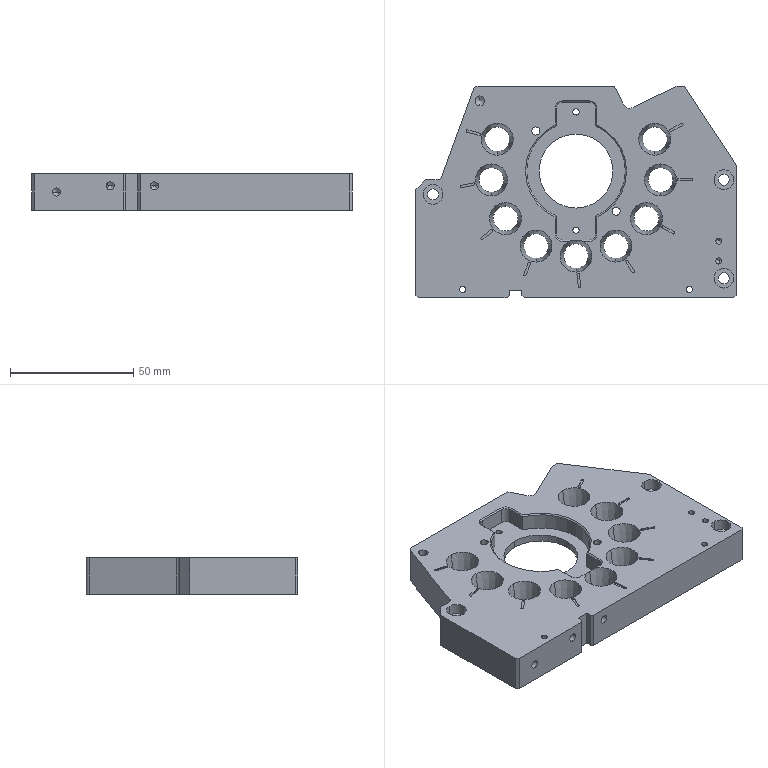NC program | NX | posted with a generic post | part box 130 x 86 x 15 mm
Lines 3983 to 5005 of 51277:
(ZLEVEL_PROFILE_1 , TOOL : D4)
N7898 T17 M6
N7900 G54
N7902 G17 G0 G90 X-13.91 Y5.2 B0. C0. S6500 M3
N7904 G43 Z30. H17
N7906 Z-0.6
N7908 G94 G1 X-14.257 Y5.8 F1650.
N7910 G3 X-14.603 Y6. R0.4
N7912 G1 X-17.
N7914 G3 X-17.5 Y5.5 R0.5
N7916 G1 Y3.103
N7918 G3 X-17.3 Y2.757 R0.4
N7920 G1 X-16.7 Y2.41
N7922 G0 X-13.91 Y5.2 Z-0.7
N7924 G1 X-14.257 Y5.8
N7926 G3 X-14.603 Y6. R0.4
N7928 G1 X-17.
N7930 G3 X-17.5 Y5.5 R0.5
N7932 G1 Y3.103
N7934 G3 X-17.3 Y2.757 R0.4
N7936 G1 X-16.7 Y2.41
N7938 G0 X-13.91 Y5.2 Z-0.8
N7940 G1 X-14.257 Y5.8
N7942 G3 X-14.603 Y6. R0.4
N7944 G1 X-17.
N7946 G3 X-17.5 Y5.5 R0.5
N7948 G1 Y3.103
N7950 G3 X-17.3 Y2.757 R0.4
N7952 G1 X-16.7 Y2.41
N7954 G0 X-13.91 Y5.2 Z-0.9
N7956 G1 X-14.257 Y5.8
N7958 G3 X-14.603 Y6. R0.4
N7960 G1 X-17.
N7962 G3 X-17.5 Y5.5 R0.5
N7964 G1 Y3.103
N7966 G3 X-17.3 Y2.757 R0.4
N7968 G1 X-16.7 Y2.41
N7970 G0 X-13.91 Y5.2 Z-1.
N7972 G1 X-14.257 Y5.8
N7974 G3 X-14.603 Y6. R0.4
N7976 G1 X-17.
N7978 G3 X-17.5 Y5.5 R0.5
N7980 G1 Y3.103
N7982 G3 X-17.3 Y2.757 R0.4
N7984 G1 X-16.7 Y2.41
N7986 G0 X-13.91 Y5.2 Z-1.1
N7988 G1 X-14.257 Y5.8
N7990 G3 X-14.603 Y6. R0.4
N7992 G1 X-17.
N7994 G3 X-17.5 Y5.5 R0.5
N7996 G1 Y3.103
N7998 G3 X-17.3 Y2.757 R0.4
N8000 G1 X-16.7 Y2.41
N8002 G0 X-13.91 Y5.2 Z-1.2
N8004 G1 X-14.257 Y5.8
N8006 G3 X-14.603 Y6. R0.4
N8008 G1 X-17.
N8010 G3 X-17.5 Y5.5 R0.5
N8012 G1 Y3.103
N8014 G3 X-17.3 Y2.757 R0.4
N8016 G1 X-16.7 Y2.41
N8018 G0 X-13.91 Y5.2 Z-1.3
N8020 G1 X-14.257 Y5.8
N8022 G3 X-14.603 Y6. R0.4
N8024 G1 X-17.
N8026 G3 X-17.5 Y5.5 R0.5
N8028 G1 Y3.103
N8030 G3 X-17.3 Y2.757 R0.4
N8032 G1 X-16.7 Y2.41
N8034 G0 X-13.91 Y5.2 Z-1.4
N8036 G1 X-14.257 Y5.8
N8038 G3 X-14.603 Y6. R0.4
N8040 G1 X-17.
N8042 G3 X-17.5 Y5.5 R0.5
N8044 G1 Y3.103
N8046 G3 X-17.3 Y2.757 R0.4
N8048 G1 X-16.7 Y2.41
N8050 G0 X-13.91 Y5.2 Z-1.5
N8052 G1 X-14.257 Y5.8
N8054 G3 X-14.603 Y6. R0.4
N8056 G1 X-17.
N8058 G3 X-17.5 Y5.5 R0.5
N8060 G1 Y3.103
N8062 G3 X-17.3 Y2.757 R0.4
N8064 G1 X-16.7 Y2.41
N8066 G0 X-13.91 Y5.2 Z-1.6
N8068 G1 X-14.257 Y5.8
N8070 G3 X-14.603 Y6. R0.4
N8072 G1 X-17.
N8074 G3 X-17.5 Y5.5 R0.5
N8076 G1 Y3.103
N8078 G3 X-17.3 Y2.757 R0.4
N8080 G1 X-16.7 Y2.41
N8082 G0 X-13.91 Y5.2 Z-1.7
N8084 G1 X-14.257 Y5.8
N8086 G3 X-14.603 Y6. R0.4
N8088 G1 X-17.
N8090 G3 X-17.5 Y5.5 R0.5
N8092 G1 Y3.103
N8094 G3 X-17.3 Y2.757 R0.4
N8096 G1 X-16.7 Y2.41
N8098 G0 X-13.91 Y5.2 Z-1.8
N8100 G1 X-14.257 Y5.8
N8102 G3 X-14.603 Y6. R0.4
N8104 G1 X-17.
N8106 G3 X-17.5 Y5.5 R0.5
N8108 G1 Y3.103
N8110 G3 X-17.3 Y2.757 R0.4
N8112 G1 X-16.7 Y2.41
N8114 G0 X-13.91 Y5.2 Z-1.9
N8116 G1 X-14.257 Y5.8
N8118 G3 X-14.603 Y6. R0.4
N8120 G1 X-17.
N8122 G3 X-17.5 Y5.5 R0.5
N8124 G1 Y3.103
N8126 G3 X-17.3 Y2.757 R0.4
N8128 G1 X-16.7 Y2.41
N8130 G0 X-13.91 Y5.2 Z-2.
N8132 G1 X-14.257 Y5.8
N8134 G3 X-14.603 Y6. R0.4
N8136 G1 X-17.
N8138 G3 X-17.5 Y5.5 R0.5
N8140 G1 Y3.103
N8142 G3 X-17.3 Y2.757 R0.4
N8144 G1 X-16.7 Y2.41
N8146 G0 X-13.91 Y5.2 Z-2.1
N8148 G1 X-14.257 Y5.8
N8150 G3 X-14.603 Y6. R0.4
N8152 G1 X-17.
N8154 G3 X-17.5 Y5.5 R0.5
N8156 G1 Y3.103
N8158 G3 X-17.3 Y2.757 R0.4
N8160 G1 X-16.7 Y2.41
N8162 G0 X-13.91 Y5.2 Z-2.2
N8164 G1 X-14.257 Y5.8
N8166 G3 X-14.603 Y6. R0.4
N8168 G1 X-17.
N8170 G3 X-17.5 Y5.5 R0.5
N8172 G1 Y3.103
N8174 G3 X-17.3 Y2.757 R0.4
N8176 G1 X-16.7 Y2.41
N8178 G0 X-13.91 Y5.2 Z-2.3
N8180 G1 X-14.257 Y5.8
N8182 G3 X-14.603 Y6. R0.4
N8184 G1 X-17.
N8186 G3 X-17.5 Y5.5 R0.5
N8188 G1 Y3.103
N8190 G3 X-17.3 Y2.757 R0.4
N8192 G1 X-16.7 Y2.41
N8194 G0 X-13.91 Y5.2 Z-2.4
N8196 G1 X-14.257 Y5.8
N8198 G3 X-14.603 Y6. R0.4
N8200 G1 X-17.
N8202 G3 X-17.5 Y5.5 R0.5
N8204 G1 Y3.103
N8206 G3 X-17.3 Y2.757 R0.4
N8208 G1 X-16.7 Y2.41
N8210 G0 X-13.91 Y5.2 Z-2.5
N8212 G1 X-14.257 Y5.8
N8214 G3 X-14.603 Y6. R0.4
N8216 G1 X-17.
N8218 G3 X-17.5 Y5.5 R0.5
N8220 G1 Y3.103
N8222 G3 X-17.3 Y2.757 R0.4
N8224 G1 X-16.7 Y2.41
N8226 G0 X-13.91 Y5.2 Z-2.6
N8228 G1 X-14.257 Y5.8
N8230 G3 X-14.603 Y6. R0.4
N8232 G1 X-17.
N8234 G3 X-17.5 Y5.5 R0.5
N8236 G1 Y3.103
N8238 G3 X-17.3 Y2.757 R0.4
N8240 G1 X-16.7 Y2.41
N8242 G0 X-13.91 Y5.2 Z-2.7
N8244 G1 X-14.257 Y5.8
N8246 G3 X-14.603 Y6. R0.4
N8248 G1 X-17.
N8250 G3 X-17.5 Y5.5 R0.5
N8252 G1 Y3.103
N8254 G3 X-17.3 Y2.757 R0.4
N8256 G1 X-16.7 Y2.41
N8258 G0 X-13.91 Y5.2 Z-2.8
N8260 G1 X-14.257 Y5.8
N8262 G3 X-14.603 Y6. R0.4
N8264 G1 X-17.
N8266 G3 X-17.5 Y5.5 R0.5
N8268 G1 Y3.103
N8270 G3 X-17.3 Y2.757 R0.4
N8272 G1 X-16.7 Y2.41
N8274 G0 X-13.91 Y5.2 Z-2.9
N8276 G1 X-14.257 Y5.8
N8278 G3 X-14.603 Y6. R0.4
N8280 G1 X-17.
N8282 G3 X-17.5 Y5.5 R0.5
N8284 G1 Y3.103
N8286 G3 X-17.3 Y2.757 R0.4
N8288 G1 X-16.7 Y2.41
N8290 G0 X-13.91 Y5.2 Z-3.
N8292 G1 X-14.257 Y5.8
N8294 G3 X-14.603 Y6. R0.4
N8296 G1 X-17.
N8298 G3 X-17.5 Y5.5 R0.5
N8300 G1 Y3.103
N8302 G3 X-17.3 Y2.757 R0.4
N8304 G1 X-16.7 Y2.41
N8306 G0 X-13.91 Y5.2 Z-3.1
N8308 G1 X-14.257 Y5.8
N8310 G3 X-14.603 Y6. R0.4
N8312 G1 X-17.
N8314 G3 X-17.5 Y5.5 R0.5
N8316 G1 Y3.103
N8318 G3 X-17.3 Y2.757 R0.4
N8320 G1 X-16.7 Y2.41
N8322 G0 X-13.91 Y5.2 Z-3.2
N8324 G1 X-14.257 Y5.8
N8326 G3 X-14.603 Y6. R0.4
N8328 G1 X-17.
N8330 G3 X-17.5 Y5.5 R0.5
N8332 G1 Y3.103
N8334 G3 X-17.3 Y2.757 R0.4
N8336 G1 X-16.7 Y2.41
N8338 G0 X-13.91 Y5.2 Z-3.3
N8340 G1 X-14.257 Y5.8
N8342 G3 X-14.603 Y6. R0.4
N8344 G1 X-17.
N8346 G3 X-17.5 Y5.5 R0.5
N8348 G1 Y3.103
N8350 G3 X-17.3 Y2.757 R0.4
N8352 G1 X-16.7 Y2.41
N8354 G0 X-13.91 Y5.2 Z-3.4
N8356 G1 X-14.257 Y5.8
N8358 G3 X-14.603 Y6. R0.4
N8360 G1 X-17.
N8362 G3 X-17.5 Y5.5 R0.5
N8364 G1 Y3.103
N8366 G3 X-17.3 Y2.757 R0.4
N8368 G1 X-16.7 Y2.41
N8370 G0 X-13.91 Y5.2 Z-3.5
N8372 G1 X-14.257 Y5.8
N8374 G3 X-14.603 Y6. R0.4
N8376 G1 X-17.
N8378 G3 X-17.5 Y5.5 R0.5
N8380 G1 Y3.103
N8382 G3 X-17.3 Y2.757 R0.4
N8384 G1 X-16.7 Y2.41
N8386 G0 X-13.91 Y5.2 Z-3.6
N8388 G1 X-14.257 Y5.8
N8390 G3 X-14.603 Y6. R0.4
N8392 G1 X-17.
N8394 G3 X-17.5 Y5.5 R0.5
N8396 G1 Y3.103
N8398 G3 X-17.3 Y2.757 R0.4
N8400 G1 X-16.7 Y2.41
N8402 G0 X-13.91 Y5.2 Z-3.7
N8404 G1 X-14.257 Y5.8
N8406 G3 X-14.603 Y6. R0.4
N8408 G1 X-17.
N8410 G3 X-17.5 Y5.5 R0.5
N8412 G1 Y3.103
N8414 G3 X-17.3 Y2.757 R0.4
N8416 G1 X-16.7 Y2.41
N8418 G0 X-13.91 Y5.2 Z-3.8
N8420 G1 X-14.257 Y5.8
N8422 G3 X-14.603 Y6. R0.4
N8424 G1 X-17.
N8426 G3 X-17.5 Y5.5 R0.5
N8428 G1 Y3.103
N8430 G3 X-17.3 Y2.757 R0.4
N8432 G1 X-16.7 Y2.41
N8434 G0 X-13.91 Y5.2 Z-3.9
N8436 G1 X-14.257 Y5.8
N8438 G3 X-14.603 Y6. R0.4
N8440 G1 X-17.
N8442 G3 X-17.5 Y5.5 R0.5
N8444 G1 Y3.103
N8446 G3 X-17.3 Y2.757 R0.4
N8448 G1 X-16.7 Y2.41
N8450 G0 X-13.91 Y5.2 Z-4.
N8452 G1 X-14.257 Y5.8
N8454 G3 X-14.603 Y6. R0.4
N8456 G1 X-17.
N8458 G3 X-17.5 Y5.5 R0.5
N8460 G1 Y3.103
N8462 G3 X-17.3 Y2.757 R0.4
N8464 G1 X-16.7 Y2.41
N8466 G0 X-13.91 Y5.2 Z-4.1
N8468 G1 X-14.257 Y5.8
N8470 G3 X-14.603 Y6. R0.4
N8472 G1 X-17.
N8474 G3 X-17.5 Y5.5 R0.5
N8476 G1 Y3.103
N8478 G3 X-17.3 Y2.757 R0.4
N8480 G1 X-16.7 Y2.41
N8482 G0 X-13.91 Y5.2 Z-4.2
N8484 G1 X-14.257 Y5.8
N8486 G3 X-14.603 Y6. R0.4
N8488 G1 X-17.
N8490 G3 X-17.5 Y5.5 R0.5
N8492 G1 Y3.103
N8494 G3 X-17.3 Y2.757 R0.4
N8496 G1 X-16.7 Y2.41
N8498 G0 X-13.91 Y5.2 Z-4.3
N8500 G1 X-14.257 Y5.8
N8502 G3 X-14.603 Y6. R0.4
N8504 G1 X-17.
N8506 G3 X-17.5 Y5.5 R0.5
N8508 G1 Y3.103
N8510 G3 X-17.3 Y2.757 R0.4
N8512 G1 X-16.7 Y2.41
N8514 G0 X-13.91 Y5.2 Z-4.4
N8516 G1 X-14.257 Y5.8
N8518 G3 X-14.603 Y6. R0.4
N8520 G1 X-17.
N8522 G3 X-17.5 Y5.5 R0.5
N8524 G1 Y3.103
N8526 G3 X-17.3 Y2.757 R0.4
N8528 G1 X-16.7 Y2.41
N8530 G0 X-13.91 Y5.2 Z-4.5
N8532 G1 X-14.257 Y5.8
N8534 G3 X-14.603 Y6. R0.4
N8536 G1 X-17.
N8538 G3 X-17.5 Y5.5 R0.5
N8540 G1 Y3.103
N8542 G3 X-17.3 Y2.757 R0.4
N8544 G1 X-16.7 Y2.41
N8546 G0 X-13.91 Y5.2 Z-4.6
N8548 G1 X-14.257 Y5.8
N8550 G3 X-14.603 Y6. R0.4
N8552 G1 X-17.
N8554 G3 X-17.5 Y5.5 R0.5
N8556 G1 Y3.103
N8558 G3 X-17.3 Y2.757 R0.4
N8560 G1 X-16.7 Y2.41
N8562 G0 X-13.91 Y5.2 Z-4.7
N8564 G1 X-14.257 Y5.8
N8566 G3 X-14.603 Y6. R0.4
N8568 G1 X-17.
N8570 G3 X-17.5 Y5.5 R0.5
N8572 G1 Y3.103
N8574 G3 X-17.3 Y2.757 R0.4
N8576 G1 X-16.7 Y2.41
N8578 G0 X-13.91 Y5.2 Z-4.8
N8580 G1 X-14.257 Y5.8
N8582 G3 X-14.603 Y6. R0.4
N8584 G1 X-17.
N8586 G3 X-17.5 Y5.5 R0.5
N8588 G1 Y3.103
N8590 G3 X-17.3 Y2.757 R0.4
N8592 G1 X-16.7 Y2.41
N8594 G0 X-13.91 Y5.2 Z-4.9
N8596 G1 X-14.257 Y5.8
N8598 G3 X-14.603 Y6. R0.4
N8600 G1 X-17.
N8602 G3 X-17.5 Y5.5 R0.5
N8604 G1 Y3.103
N8606 G3 X-17.3 Y2.757 R0.4
N8608 G1 X-16.7 Y2.41
N8610 G0 X-13.91 Y5.2 Z-5.
N8612 G1 X-14.257 Y5.8
N8614 G3 X-14.603 Y6. R0.4
N8616 G1 X-17.
N8618 G3 X-17.5 Y5.5 R0.5
N8620 G1 Y3.103
N8622 G3 X-17.3 Y2.757 R0.4
N8624 G1 X-16.7 Y2.41
N8626 G0 X-13.91 Y5.2 Z-5.1
N8628 G1 X-14.257 Y5.8
N8630 G3 X-14.603 Y6. R0.4
N8632 G1 X-17.
N8634 G3 X-17.5 Y5.5 R0.5
N8636 G1 Y3.103
N8638 G3 X-17.3 Y2.757 R0.4
N8640 G1 X-16.7 Y2.41
N8642 G0 X-13.91 Y5.2 Z-5.2
N8644 G1 X-14.257 Y5.8
N8646 G3 X-14.603 Y6. R0.4
N8648 G1 X-17.
N8650 G3 X-17.5 Y5.5 R0.5
N8652 G1 Y3.103
N8654 G3 X-17.3 Y2.757 R0.4
N8656 G1 X-16.7 Y2.41
N8658 G0 X-13.91 Y5.2 Z-5.3
N8660 G1 X-14.257 Y5.8
N8662 G3 X-14.603 Y6. R0.4
N8664 G1 X-17.
N8666 G3 X-17.5 Y5.5 R0.5
N8668 G1 Y3.103
N8670 G3 X-17.3 Y2.757 R0.4
N8672 G1 X-16.7 Y2.41
N8674 G0 X-13.91 Y5.2 Z-5.4
N8676 G1 X-14.257 Y5.8
N8678 G3 X-14.603 Y6. R0.4
N8680 G1 X-17.
N8682 G3 X-17.5 Y5.5 R0.5
N8684 G1 Y3.103
N8686 G3 X-17.3 Y2.757 R0.4
N8688 G1 X-16.7 Y2.41
N8690 G0 X-13.91 Y5.2 Z-5.5
N8692 G1 X-14.257 Y5.8
N8694 G3 X-14.603 Y6. R0.4
N8696 G1 X-17.
N8698 G3 X-17.5 Y5.5 R0.5
N8700 G1 Y3.103
N8702 G3 X-17.3 Y2.757 R0.4
N8704 G1 X-16.7 Y2.41
N8706 G0 X-13.91 Y5.2 Z-5.6
N8708 G1 X-14.257 Y5.8
N8710 G3 X-14.603 Y6. R0.4
N8712 G1 X-17.
N8714 G3 X-17.5 Y5.5 R0.5
N8716 G1 Y3.103
N8718 G3 X-17.3 Y2.757 R0.4
N8720 G1 X-16.7 Y2.41
N8722 G0 X-13.91 Y5.2 Z-5.7
N8724 G1 X-14.257 Y5.8
N8726 G3 X-14.603 Y6. R0.4
N8728 G1 X-17.
N8730 G3 X-17.5 Y5.5 R0.5
N8732 G1 Y3.103
N8734 G3 X-17.3 Y2.757 R0.4
N8736 G1 X-16.7 Y2.41
N8738 G0 X-13.91 Y5.2 Z-5.8
N8740 G1 X-14.257 Y5.8
N8742 G3 X-14.603 Y6. R0.4
N8744 G1 X-17.
N8746 G3 X-17.5 Y5.5 R0.5
N8748 G1 Y3.103
N8750 G3 X-17.3 Y2.757 R0.4
N8752 G1 X-16.7 Y2.41
N8754 G0 X-13.91 Y5.2 Z-5.9
N8756 G1 X-14.257 Y5.8
N8758 G3 X-14.603 Y6. R0.4
N8760 G1 X-17.
N8762 G3 X-17.5 Y5.5 R0.5
N8764 G1 Y3.103
N8766 G3 X-17.3 Y2.757 R0.4
N8768 G1 X-16.7 Y2.41
N8770 G0 X-13.91 Y5.2 Z-6.
N8772 G1 X-14.257 Y5.8
N8774 G3 X-14.603 Y6. R0.4
N8776 G1 X-17.
N8778 G3 X-17.5 Y5.5 R0.5
N8780 G1 Y3.103
N8782 G3 X-17.3 Y2.757 R0.4
N8784 G1 X-16.7 Y2.41
N8786 G0 X-13.91 Y5.2 Z-6.1
N8788 G1 X-14.257 Y5.8
N8790 G3 X-14.603 Y6. R0.4
N8792 G1 X-17.
N8794 G3 X-17.5 Y5.5 R0.5
N8796 G1 Y3.103
N8798 G3 X-17.3 Y2.757 R0.4
N8800 G1 X-16.7 Y2.41
N8802 G0 X-13.91 Y5.2 Z-6.2
N8804 G1 X-14.257 Y5.8
N8806 G3 X-14.603 Y6. R0.4
N8808 G1 X-17.
N8810 G3 X-17.5 Y5.5 R0.5
N8812 G1 Y3.103
N8814 G3 X-17.3 Y2.757 R0.4
N8816 G1 X-16.7 Y2.41
N8818 G0 X-13.91 Y5.2 Z-6.3
N8820 G1 X-14.257 Y5.8
N8822 G3 X-14.603 Y6. R0.4
N8824 G1 X-17.
N8826 G3 X-17.5 Y5.5 R0.5
N8828 G1 Y3.103
N8830 G3 X-17.3 Y2.757 R0.4
N8832 G1 X-16.7 Y2.41
N8834 G0 X-13.91 Y5.2 Z-6.4
N8836 G1 X-14.257 Y5.8
N8838 G3 X-14.603 Y6. R0.4
N8840 G1 X-17.
N8842 G3 X-17.5 Y5.5 R0.5
N8844 G1 Y3.103
N8846 G3 X-17.3 Y2.757 R0.4
N8848 G1 X-16.7 Y2.41
N8850 G0 X-13.91 Y5.2 Z-6.5
N8852 G1 X-14.257 Y5.8
N8854 G3 X-14.603 Y6. R0.4
N8856 G1 X-17.
N8858 G3 X-17.5 Y5.5 R0.5
N8860 G1 Y3.103
N8862 G3 X-17.3 Y2.757 R0.4
N8864 G1 X-16.7 Y2.41
N8866 G0 X-13.91 Y5.2 Z-6.6
N8868 G1 X-14.257 Y5.8
N8870 G3 X-14.603 Y6. R0.4
N8872 G1 X-17.
N8874 G3 X-17.5 Y5.5 R0.5
N8876 G1 Y3.103
N8878 G3 X-17.3 Y2.757 R0.4
N8880 G1 X-16.7 Y2.41
N8882 G0 X-13.91 Y5.2 Z-6.7
N8884 G1 X-14.257 Y5.8
N8886 G3 X-14.603 Y6. R0.4
N8888 G1 X-17.
N8890 G3 X-17.5 Y5.5 R0.5
N8892 G1 Y3.103
N8894 G3 X-17.3 Y2.757 R0.4
N8896 G1 X-16.7 Y2.41
N8898 G0 X-13.91 Y5.2 Z-6.8
N8900 G1 X-14.257 Y5.8
N8902 G3 X-14.603 Y6. R0.4
N8904 G1 X-17.
N8906 G3 X-17.5 Y5.5 R0.5
N8908 G1 Y3.103
N8910 G3 X-17.3 Y2.757 R0.4
N8912 G1 X-16.7 Y2.41
N8914 G0 X-13.91 Y5.2 Z-6.9
N8916 G1 X-14.257 Y5.8
N8918 G3 X-14.603 Y6. R0.4
N8920 G1 X-17.
N8922 G3 X-17.5 Y5.5 R0.5
N8924 G1 Y3.103
N8926 G3 X-17.3 Y2.757 R0.4
N8928 G1 X-16.7 Y2.41
N8930 G0 X-13.91 Y5.2 Z-7.
N8932 G1 X-14.257 Y5.8
N8934 G3 X-14.603 Y6. R0.4
N8936 G1 X-17.
N8938 G3 X-17.5 Y5.5 R0.5
N8940 G1 Y3.103
N8942 G3 X-17.3 Y2.757 R0.4
N8944 G1 X-16.7 Y2.41
N8946 G0 Z30.
N8948 Y-2.41
N8950 Z-0.6
N8952 G1 X-17.3 Y-2.757
N8954 G3 X-17.5 Y-3.103 R0.4
N8956 G1 Y-5.5
N8958 G3 X-17. Y-6. R0.5
N8960 G1 X-14.603
N8962 G3 X-14.257 Y-5.8 R0.4
N8964 G1 X-13.91 Y-5.2
N8966 G0 X-16.7 Y-2.41 Z-0.7
N8968 G1 X-17.3 Y-2.757
N8970 G3 X-17.5 Y-3.103 R0.4
N8972 G1 Y-5.5
N8974 G3 X-17. Y-6. R0.5
N8976 G1 X-14.603
N8978 G3 X-14.257 Y-5.8 R0.4
N8980 G1 X-13.91 Y-5.2
N8982 G0 X-16.7 Y-2.41 Z-0.8
N8984 G1 X-17.3 Y-2.757
N8986 G3 X-17.5 Y-3.103 R0.4
N8988 G1 Y-5.5
N8990 G3 X-17. Y-6. R0.5
N8992 G1 X-14.603
N8994 G3 X-14.257 Y-5.8 R0.4
N8996 G1 X-13.91 Y-5.2
N8998 G0 X-16.7 Y-2.41 Z-0.9
N9000 G1 X-17.3 Y-2.757
N9002 G3 X-17.5 Y-3.103 R0.4
N9004 G1 Y-5.5
N9006 G3 X-17. Y-6. R0.5
N9008 G1 X-14.603
N9010 G3 X-14.257 Y-5.8 R0.4
N9012 G1 X-13.91 Y-5.2
N9014 G0 X-16.7 Y-2.41 Z-1.
N9016 G1 X-17.3 Y-2.757
N9018 G3 X-17.5 Y-3.103 R0.4
N9020 G1 Y-5.5
N9022 G3 X-17. Y-6. R0.5
N9024 G1 X-14.603
N9026 G3 X-14.257 Y-5.8 R0.4
N9028 G1 X-13.91 Y-5.2
N9030 G0 X-16.7 Y-2.41 Z-1.1
N9032 G1 X-17.3 Y-2.757
N9034 G3 X-17.5 Y-3.103 R0.4
N9036 G1 Y-5.5
N9038 G3 X-17. Y-6. R0.5
N9040 G1 X-14.603
N9042 G3 X-14.257 Y-5.8 R0.4
N9044 G1 X-13.91 Y-5.2
N9046 G0 X-16.7 Y-2.41 Z-1.2
N9048 G1 X-17.3 Y-2.757
N9050 G3 X-17.5 Y-3.103 R0.4
N9052 G1 Y-5.5
N9054 G3 X-17. Y-6. R0.5
N9056 G1 X-14.603
N9058 G3 X-14.257 Y-5.8 R0.4
N9060 G1 X-13.91 Y-5.2
N9062 G0 X-16.7 Y-2.41 Z-1.3
N9064 G1 X-17.3 Y-2.757
N9066 G3 X-17.5 Y-3.103 R0.4
N9068 G1 Y-5.5
N9070 G3 X-17. Y-6. R0.5
N9072 G1 X-14.603
N9074 G3 X-14.257 Y-5.8 R0.4
N9076 G1 X-13.91 Y-5.2
N9078 G0 X-16.7 Y-2.41 Z-1.4
N9080 G1 X-17.3 Y-2.757
N9082 G3 X-17.5 Y-3.103 R0.4
N9084 G1 Y-5.5
N9086 G3 X-17. Y-6. R0.5
N9088 G1 X-14.603
N9090 G3 X-14.257 Y-5.8 R0.4
N9092 G1 X-13.91 Y-5.2
N9094 G0 X-16.7 Y-2.41 Z-1.5
N9096 G1 X-17.3 Y-2.757
N9098 G3 X-17.5 Y-3.103 R0.4
N9100 G1 Y-5.5
N9102 G3 X-17. Y-6. R0.5
N9104 G1 X-14.603
N9106 G3 X-14.257 Y-5.8 R0.4
N9108 G1 X-13.91 Y-5.2
N9110 G0 X-16.7 Y-2.41 Z-1.6
N9112 G1 X-17.3 Y-2.757
N9114 G3 X-17.5 Y-3.103 R0.4
N9116 G1 Y-5.5
N9118 G3 X-17. Y-6. R0.5
N9120 G1 X-14.603
N9122 G3 X-14.257 Y-5.8 R0.4
N9124 G1 X-13.91 Y-5.2
N9126 G0 X-16.7 Y-2.41 Z-1.7
N9128 G1 X-17.3 Y-2.757
N9130 G3 X-17.5 Y-3.103 R0.4
N9132 G1 Y-5.5
N9134 G3 X-17. Y-6. R0.5
N9136 G1 X-14.603
N9138 G3 X-14.257 Y-5.8 R0.4
N9140 G1 X-13.91 Y-5.2
N9142 G0 X-16.7 Y-2.41 Z-1.8
N9144 G1 X-17.3 Y-2.757
N9146 G3 X-17.5 Y-3.103 R0.4
N9148 G1 Y-5.5
N9150 G3 X-17. Y-6. R0.5
N9152 G1 X-14.603
N9154 G3 X-14.257 Y-5.8 R0.4
N9156 G1 X-13.91 Y-5.2
N9158 G0 X-16.7 Y-2.41 Z-1.9
N9160 G1 X-17.3 Y-2.757
N9162 G3 X-17.5 Y-3.103 R0.4
N9164 G1 Y-5.5
N9166 G3 X-17. Y-6. R0.5
N9168 G1 X-14.603
N9170 G3 X-14.257 Y-5.8 R0.4
N9172 G1 X-13.91 Y-5.2
N9174 G0 X-16.7 Y-2.41 Z-2.
N9176 G1 X-17.3 Y-2.757
N9178 G3 X-17.5 Y-3.103 R0.4
N9180 G1 Y-5.5
N9182 G3 X-17. Y-6. R0.5
N9184 G1 X-14.603
N9186 G3 X-14.257 Y-5.8 R0.4
N9188 G1 X-13.91 Y-5.2
N9190 G0 X-16.7 Y-2.41 Z-2.1
N9192 G1 X-17.3 Y-2.757
N9194 G3 X-17.5 Y-3.103 R0.4
N9196 G1 Y-5.5
N9198 G3 X-17. Y-6. R0.5
N9200 G1 X-14.603
N9202 G3 X-14.257 Y-5.8 R0.4
N9204 G1 X-13.91 Y-5.2
N9206 G0 X-16.7 Y-2.41 Z-2.2
N9208 G1 X-17.3 Y-2.757
N9210 G3 X-17.5 Y-3.103 R0.4
N9212 G1 Y-5.5
N9214 G3 X-17. Y-6. R0.5
N9216 G1 X-14.603
N9218 G3 X-14.257 Y-5.8 R0.4
N9220 G1 X-13.91 Y-5.2
N9222 G0 X-16.7 Y-2.41 Z-2.3
N9224 G1 X-17.3 Y-2.757
N9226 G3 X-17.5 Y-3.103 R0.4
N9228 G1 Y-5.5
N9230 G3 X-17. Y-6. R0.5
N9232 G1 X-14.603
N9234 G3 X-14.257 Y-5.8 R0.4
N9236 G1 X-13.91 Y-5.2
N9238 G0 X-16.7 Y-2.41 Z-2.4
N9240 G1 X-17.3 Y-2.757
N9242 G3 X-17.5 Y-3.103 R0.4
N9244 G1 Y-5.5
N9246 G3 X-17. Y-6. R0.5
N9248 G1 X-14.603
N9250 G3 X-14.257 Y-5.8 R0.4
N9252 G1 X-13.91 Y-5.2
N9254 G0 X-16.7 Y-2.41 Z-2.5
N9256 G1 X-17.3 Y-2.757
N9258 G3 X-17.5 Y-3.103 R0.4
N9260 G1 Y-5.5
N9262 G3 X-17. Y-6. R0.5
N9264 G1 X-14.603
N9266 G3 X-14.257 Y-5.8 R0.4
N9268 G1 X-13.91 Y-5.2
N9270 G0 X-16.7 Y-2.41 Z-2.6
N9272 G1 X-17.3 Y-2.757
N9274 G3 X-17.5 Y-3.103 R0.4
N9276 G1 Y-5.5
N9278 G3 X-17. Y-6. R0.5
N9280 G1 X-14.603
N9282 G3 X-14.257 Y-5.8 R0.4
N9284 G1 X-13.91 Y-5.2
N9286 G0 X-16.7 Y-2.41 Z-2.7
N9288 G1 X-17.3 Y-2.757
N9290 G3 X-17.5 Y-3.103 R0.4
N9292 G1 Y-5.5
N9294 G3 X-17. Y-6. R0.5
N9296 G1 X-14.603
N9298 G3 X-14.257 Y-5.8 R0.4
N9300 G1 X-13.91 Y-5.2
N9302 G0 X-16.7 Y-2.41 Z-2.8
N9304 G1 X-17.3 Y-2.757
N9306 G3 X-17.5 Y-3.103 R0.4
N9308 G1 Y-5.5
N9310 G3 X-17. Y-6. R0.5
N9312 G1 X-14.603
N9314 G3 X-14.257 Y-5.8 R0.4
N9316 G1 X-13.91 Y-5.2
N9318 G0 X-16.7 Y-2.41 Z-2.9
N9320 G1 X-17.3 Y-2.757
N9322 G3 X-17.5 Y-3.103 R0.4
N9324 G1 Y-5.5
N9326 G3 X-17. Y-6. R0.5
N9328 G1 X-14.603
N9330 G3 X-14.257 Y-5.8 R0.4
N9332 G1 X-13.91 Y-5.2
N9334 G0 X-16.7 Y-2.41 Z-3.
N9336 G1 X-17.3 Y-2.757
N9338 G3 X-17.5 Y-3.103 R0.4
N9340 G1 Y-5.5
N9342 G3 X-17. Y-6. R0.5
N9344 G1 X-14.603
N9346 G3 X-14.257 Y-5.8 R0.4
N9348 G1 X-13.91 Y-5.2
N9350 G0 X-16.7 Y-2.41 Z-3.1
N9352 G1 X-17.3 Y-2.757
N9354 G3 X-17.5 Y-3.103 R0.4
N9356 G1 Y-5.5
N9358 G3 X-17. Y-6. R0.5
N9360 G1 X-14.603
N9362 G3 X-14.257 Y-5.8 R0.4
N9364 G1 X-13.91 Y-5.2
N9366 G0 X-16.7 Y-2.41 Z-3.2
N9368 G1 X-17.3 Y-2.757
N9370 G3 X-17.5 Y-3.103 R0.4
N9372 G1 Y-5.5
N9374 G3 X-17. Y-6. R0.5
N9376 G1 X-14.603
N9378 G3 X-14.257 Y-5.8 R0.4
N9380 G1 X-13.91 Y-5.2
N9382 G0 X-16.7 Y-2.41 Z-3.3
N9384 G1 X-17.3 Y-2.757
N9386 G3 X-17.5 Y-3.103 R0.4
N9388 G1 Y-5.5
N9390 G3 X-17. Y-6. R0.5
N9392 G1 X-14.603
N9394 G3 X-14.257 Y-5.8 R0.4
N9396 G1 X-13.91 Y-5.2
N9398 G0 X-16.7 Y-2.41 Z-3.4
N9400 G1 X-17.3 Y-2.757
N9402 G3 X-17.5 Y-3.103 R0.4
N9404 G1 Y-5.5
N9406 G3 X-17. Y-6. R0.5
N9408 G1 X-14.603
N9410 G3 X-14.257 Y-5.8 R0.4
N9412 G1 X-13.91 Y-5.2
N9414 G0 X-16.7 Y-2.41 Z-3.5
N9416 G1 X-17.3 Y-2.757
N9418 G3 X-17.5 Y-3.103 R0.4
N9420 G1 Y-5.5
N9422 G3 X-17. Y-6. R0.5
N9424 G1 X-14.603
N9426 G3 X-14.257 Y-5.8 R0.4
N9428 G1 X-13.91 Y-5.2
N9430 G0 X-16.7 Y-2.41 Z-3.6
N9432 G1 X-17.3 Y-2.757
N9434 G3 X-17.5 Y-3.103 R0.4
N9436 G1 Y-5.5
N9438 G3 X-17. Y-6. R0.5
N9440 G1 X-14.603
N9442 G3 X-14.257 Y-5.8 R0.4
N9444 G1 X-13.91 Y-5.2
N9446 G0 X-16.7 Y-2.41 Z-3.7
N9448 G1 X-17.3 Y-2.757
N9450 G3 X-17.5 Y-3.103 R0.4
N9452 G1 Y-5.5
N9454 G3 X-17. Y-6. R0.5
N9456 G1 X-14.603
N9458 G3 X-14.257 Y-5.8 R0.4
N9460 G1 X-13.91 Y-5.2
N9462 G0 X-16.7 Y-2.41 Z-3.8
N9464 G1 X-17.3 Y-2.757
N9466 G3 X-17.5 Y-3.103 R0.4
N9468 G1 Y-5.5
N9470 G3 X-17. Y-6. R0.5
N9472 G1 X-14.603
N9474 G3 X-14.257 Y-5.8 R0.4
N9476 G1 X-13.91 Y-5.2
N9478 G0 X-16.7 Y-2.41 Z-3.9
N9480 G1 X-17.3 Y-2.757
N9482 G3 X-17.5 Y-3.103 R0.4
N9484 G1 Y-5.5
N9486 G3 X-17. Y-6. R0.5
N9488 G1 X-14.603
N9490 G3 X-14.257 Y-5.8 R0.4
N9492 G1 X-13.91 Y-5.2
N9494 G0 X-16.7 Y-2.41 Z-4.
N9496 G1 X-17.3 Y-2.757
N9498 G3 X-17.5 Y-3.103 R0.4
N9500 G1 Y-5.5
N9502 G3 X-17. Y-6. R0.5
N9504 G1 X-14.603
N9506 G3 X-14.257 Y-5.8 R0.4
N9508 G1 X-13.91 Y-5.2
N9510 G0 X-16.7 Y-2.41 Z-4.1
N9512 G1 X-17.3 Y-2.757
N9514 G3 X-17.5 Y-3.103 R0.4
N9516 G1 Y-5.5
N9518 G3 X-17. Y-6. R0.5
N9520 G1 X-14.603
N9522 G3 X-14.257 Y-5.8 R0.4
N9524 G1 X-13.91 Y-5.2
N9526 G0 X-16.7 Y-2.41 Z-4.2
N9528 G1 X-17.3 Y-2.757
N9530 G3 X-17.5 Y-3.103 R0.4
N9532 G1 Y-5.5
N9534 G3 X-17. Y-6. R0.5
N9536 G1 X-14.603
N9538 G3 X-14.257 Y-5.8 R0.4
N9540 G1 X-13.91 Y-5.2
N9542 G0 X-16.7 Y-2.41 Z-4.3
N9544 G1 X-17.3 Y-2.757
N9546 G3 X-17.5 Y-3.103 R0.4
N9548 G1 Y-5.5
N9550 G3 X-17. Y-6. R0.5
N9552 G1 X-14.603
N9554 G3 X-14.257 Y-5.8 R0.4
N9556 G1 X-13.91 Y-5.2
N9558 G0 X-16.7 Y-2.41 Z-4.4
N9560 G1 X-17.3 Y-2.757
N9562 G3 X-17.5 Y-3.103 R0.4
N9564 G1 Y-5.5
N9566 G3 X-17. Y-6. R0.5
N9568 G1 X-14.603
N9570 G3 X-14.257 Y-5.8 R0.4
N9572 G1 X-13.91 Y-5.2
N9574 G0 X-16.7 Y-2.41 Z-4.5
N9576 G1 X-17.3 Y-2.757
N9578 G3 X-17.5 Y-3.103 R0.4
N9580 G1 Y-5.5
N9582 G3 X-17. Y-6. R0.5
N9584 G1 X-14.603
N9586 G3 X-14.257 Y-5.8 R0.4
N9588 G1 X-13.91 Y-5.2
N9590 G0 X-16.7 Y-2.41 Z-4.6
N9592 G1 X-17.3 Y-2.757
N9594 G3 X-17.5 Y-3.103 R0.4
N9596 G1 Y-5.5
N9598 G3 X-17. Y-6. R0.5
N9600 G1 X-14.603
N9602 G3 X-14.257 Y-5.8 R0.4
N9604 G1 X-13.91 Y-5.2
N9606 G0 X-16.7 Y-2.41 Z-4.7
N9608 G1 X-17.3 Y-2.757
N9610 G3 X-17.5 Y-3.103 R0.4
N9612 G1 Y-5.5
N9614 G3 X-17. Y-6. R0.5
N9616 G1 X-14.603
N9618 G3 X-14.257 Y-5.8 R0.4
N9620 G1 X-13.91 Y-5.2
N9622 G0 X-16.7 Y-2.41 Z-4.8
N9624 G1 X-17.3 Y-2.757
N9626 G3 X-17.5 Y-3.103 R0.4
N9628 G1 Y-5.5
N9630 G3 X-17. Y-6. R0.5
N9632 G1 X-14.603
N9634 G3 X-14.257 Y-5.8 R0.4
N9636 G1 X-13.91 Y-5.2
N9638 G0 X-16.7 Y-2.41 Z-4.9
N9640 G1 X-17.3 Y-2.757
N9642 G3 X-17.5 Y-3.103 R0.4
N9644 G1 Y-5.5
N9646 G3 X-17. Y-6. R0.5
N9648 G1 X-14.603
N9650 G3 X-14.257 Y-5.8 R0.4
N9652 G1 X-13.91 Y-5.2
N9654 G0 X-16.7 Y-2.41 Z-5.
N9656 G1 X-17.3 Y-2.757
N9658 G3 X-17.5 Y-3.103 R0.4
N9660 G1 Y-5.5
N9662 G3 X-17. Y-6. R0.5
N9664 G1 X-14.603
N9666 G3 X-14.257 Y-5.8 R0.4
N9668 G1 X-13.91 Y-5.2
N9670 G0 X-16.7 Y-2.41 Z-5.1
N9672 G1 X-17.3 Y-2.757
N9674 G3 X-17.5 Y-3.103 R0.4
N9676 G1 Y-5.5
N9678 G3 X-17. Y-6. R0.5
N9680 G1 X-14.603
N9682 G3 X-14.257 Y-5.8 R0.4
N9684 G1 X-13.91 Y-5.2
N9686 G0 X-16.7 Y-2.41 Z-5.2
N9688 G1 X-17.3 Y-2.757
N9690 G3 X-17.5 Y-3.103 R0.4
N9692 G1 Y-5.5
N9694 G3 X-17. Y-6. R0.5
N9696 G1 X-14.603
N9698 G3 X-14.257 Y-5.8 R0.4
N9700 G1 X-13.91 Y-5.2
N9702 G0 X-16.7 Y-2.41 Z-5.3
N9704 G1 X-17.3 Y-2.757
N9706 G3 X-17.5 Y-3.103 R0.4
N9708 G1 Y-5.5
N9710 G3 X-17. Y-6. R0.5
N9712 G1 X-14.603
N9714 G3 X-14.257 Y-5.8 R0.4
N9716 G1 X-13.91 Y-5.2
N9718 G0 X-16.7 Y-2.41 Z-5.4
N9720 G1 X-17.3 Y-2.757
N9722 G3 X-17.5 Y-3.103 R0.4
N9724 G1 Y-5.5
N9726 G3 X-17. Y-6. R0.5
N9728 G1 X-14.603
N9730 G3 X-14.257 Y-5.8 R0.4
N9732 G1 X-13.91 Y-5.2
N9734 G0 X-16.7 Y-2.41 Z-5.5
N9736 G1 X-17.3 Y-2.757
N9738 G3 X-17.5 Y-3.103 R0.4
N9740 G1 Y-5.5
N9742 G3 X-17. Y-6. R0.5
N9744 G1 X-14.603
N9746 G3 X-14.257 Y-5.8 R0.4
N9748 G1 X-13.91 Y-5.2
N9750 G0 X-16.7 Y-2.41 Z-5.6
N9752 G1 X-17.3 Y-2.757
N9754 G3 X-17.5 Y-3.103 R0.4
N9756 G1 Y-5.5
N9758 G3 X-17. Y-6. R0.5
N9760 G1 X-14.603
N9762 G3 X-14.257 Y-5.8 R0.4
N9764 G1 X-13.91 Y-5.2
N9766 G0 X-16.7 Y-2.41 Z-5.7
N9768 G1 X-17.3 Y-2.757
N9770 G3 X-17.5 Y-3.103 R0.4
N9772 G1 Y-5.5
N9774 G3 X-17. Y-6. R0.5
N9776 G1 X-14.603
N9778 G3 X-14.257 Y-5.8 R0.4
N9780 G1 X-13.91 Y-5.2
N9782 G0 X-16.7 Y-2.41 Z-5.8
N9784 G1 X-17.3 Y-2.757
N9786 G3 X-17.5 Y-3.103 R0.4
N9788 G1 Y-5.5
N9790 G3 X-17. Y-6. R0.5
N9792 G1 X-14.603
N9794 G3 X-14.257 Y-5.8 R0.4
N9796 G1 X-13.91 Y-5.2
N9798 G0 X-16.7 Y-2.41 Z-5.9
N9800 G1 X-17.3 Y-2.757
N9802 G3 X-17.5 Y-3.103 R0.4
N9804 G1 Y-5.5
N9806 G3 X-17. Y-6. R0.5
N9808 G1 X-14.603
N9810 G3 X-14.257 Y-5.8 R0.4
N9812 G1 X-13.91 Y-5.2
N9814 G0 X-16.7 Y-2.41 Z-6.
N9816 G1 X-17.3 Y-2.757
N9818 G3 X-17.5 Y-3.103 R0.4
N9820 G1 Y-5.5
N9822 G3 X-17. Y-6. R0.5
N9824 G1 X-14.603
N9826 G3 X-14.257 Y-5.8 R0.4
N9828 G1 X-13.91 Y-5.2
N9830 G0 X-16.7 Y-2.41 Z-6.1
N9832 G1 X-17.3 Y-2.757
N9834 G3 X-17.5 Y-3.103 R0.4
N9836 G1 Y-5.5
N9838 G3 X-17. Y-6. R0.5
N9840 G1 X-14.603
N9842 G3 X-14.257 Y-5.8 R0.4
N9844 G1 X-13.91 Y-5.2
N9846 G0 X-16.7 Y-2.41 Z-6.2
N9848 G1 X-17.3 Y-2.757
N9850 G3 X-17.5 Y-3.103 R0.4
N9852 G1 Y-5.5
N9854 G3 X-17. Y-6. R0.5
N9856 G1 X-14.603
N9858 G3 X-14.257 Y-5.8 R0.4
N9860 G1 X-13.91 Y-5.2
N9862 G0 X-16.7 Y-2.41 Z-6.3
N9864 G1 X-17.3 Y-2.757
N9866 G3 X-17.5 Y-3.103 R0.4
N9868 G1 Y-5.5
N9870 G3 X-17. Y-6. R0.5
N9872 G1 X-14.603
N9874 G3 X-14.257 Y-5.8 R0.4
N9876 G1 X-13.91 Y-5.2
N9878 G0 X-16.7 Y-2.41 Z-6.4
N9880 G1 X-17.3 Y-2.757
N9882 G3 X-17.5 Y-3.103 R0.4
N9884 G1 Y-5.5
N9886 G3 X-17. Y-6. R0.5
N9888 G1 X-14.603
N9890 G3 X-14.257 Y-5.8 R0.4
N9892 G1 X-13.91 Y-5.2
N9894 G0 X-16.7 Y-2.41 Z-6.5
N9896 G1 X-17.3 Y-2.757
N9898 G3 X-17.5 Y-3.103 R0.4
N9900 G1 Y-5.5
N9902 G3 X-17. Y-6. R0.5
N9904 G1 X-14.603
N9906 G3 X-14.257 Y-5.8 R0.4
N9908 G1 X-13.91 Y-5.2
N9910 G0 X-16.7 Y-2.41 Z-6.6
N9912 G1 X-17.3 Y-2.757
N9914 G3 X-17.5 Y-3.103 R0.4
N9916 G1 Y-5.5
N9918 G3 X-17. Y-6. R0.5
N9920 G1 X-14.603
N9922 G3 X-14.257 Y-5.8 R0.4
N9924 G1 X-13.91 Y-5.2
N9926 G0 X-16.7 Y-2.41 Z-6.7
N9928 G1 X-17.3 Y-2.757
N9930 G3 X-17.5 Y-3.103 R0.4
N9932 G1 Y-5.5
N9934 G3 X-17. Y-6. R0.5
N9936 G1 X-14.603